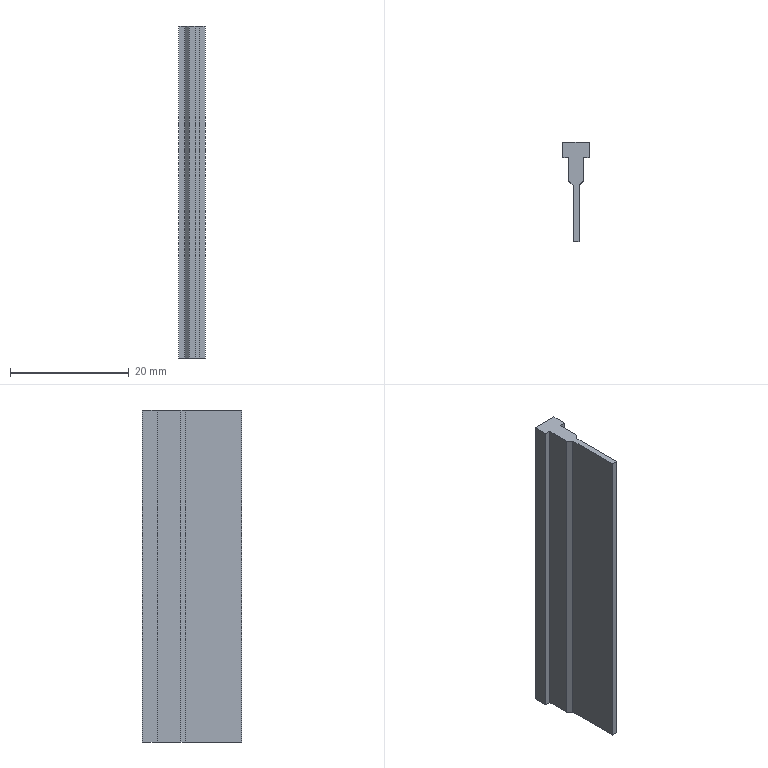Part | NX | features BREP 2 | 2 solids | 28 faces | box 4.458 x 16.702 x 56 mm | volume 3550 mm3 | plane 28
STEP:
#1=CARTESIAN_POINT('',(1.229,1.86,-4.));
#2=VERTEX_POINT('',#1);
#3=CARTESIAN_POINT('',(1.229,1.86,52.));
#4=VERTEX_POINT('',#3);
#5=CARTESIAN_POINT('',(1.229,1.86,0.));
#6=DIRECTION('',(0.,0.,1.));
#7=VECTOR('',#6,1000.);
#8=LINE('',#5,#7);
#9=EDGE_CURVE('',#2,#4,#8,.T.);
#10=ORIENTED_EDGE('',*,*,#9,.T.);
#11=CARTESIAN_POINT('',(0.521,1.152,52.));
#12=VERTEX_POINT('',#11);
#13=CARTESIAN_POINT('',(1.229,1.86,52.));
#14=DIRECTION('',(0.7071,0.7071,0.));
#15=VECTOR('',#14,1000.);
#16=LINE('',#13,#15);
#17=EDGE_CURVE('',#12,#4,#16,.T.);
#18=ORIENTED_EDGE('',*,*,#17,.F.);
#19=CARTESIAN_POINT('',(0.521,1.152,-4.));
#20=VERTEX_POINT('',#19);
#21=CARTESIAN_POINT('',(0.521,1.152,0.));
#22=DIRECTION('',(0.,0.,1.));
#23=VECTOR('',#22,1000.);
#24=LINE('',#21,#23);
#25=EDGE_CURVE('',#20,#12,#24,.T.);
#26=ORIENTED_EDGE('',*,*,#25,.F.);
#27=CARTESIAN_POINT('',(1.229,1.86,-4.));
#28=DIRECTION('',(0.7071,0.7071,0.));
#29=VECTOR('',#28,1000.);
#30=LINE('',#27,#29);
#31=EDGE_CURVE('',#20,#2,#30,.T.);
#32=ORIENTED_EDGE('',*,*,#31,.T.);
#33=EDGE_LOOP('',(#10,#18,#26,#32));
#34=FACE_BOUND('',#33,.T.);
#35=CARTESIAN_POINT('',(1.229,1.86,0.));
#36=DIRECTION('',(-0.7071,0.7071,0.));
#37=DIRECTION('',(0.7071,0.7071,0.));
#38=AXIS2_PLACEMENT_3D('',#35,#36,#37);
#39=PLANE('',#38);
#40=ADVANCED_FACE('',(#34),#39,.F.);
#41=CARTESIAN_POINT('',(0.521,-8.351,-4.));
#42=VERTEX_POINT('',#41);
#43=CARTESIAN_POINT('',(0.521,-8.351,52.));
#44=VERTEX_POINT('',#43);
#45=CARTESIAN_POINT('',(0.521,-8.351,0.));
#46=DIRECTION('',(0.,0.,1.));
#47=VECTOR('',#46,1000.);
#48=LINE('',#45,#47);
#49=EDGE_CURVE('',#42,#44,#48,.T.);
#50=ORIENTED_EDGE('',*,*,#49,.F.);
#51=CARTESIAN_POINT('',(0.521,-22.649,-4.));
#52=DIRECTION('',(0.,1.,0.));
#53=VECTOR('',#52,1000.);
#54=LINE('',#51,#53);
#55=EDGE_CURVE('',#42,#20,#54,.T.);
#56=ORIENTED_EDGE('',*,*,#55,.T.);
#57=ORIENTED_EDGE('',*,*,#25,.T.);
#58=CARTESIAN_POINT('',(0.521,-22.649,52.));
#59=DIRECTION('',(0.,1.,0.));
#60=VECTOR('',#59,1000.);
#61=LINE('',#58,#60);
#62=EDGE_CURVE('',#44,#12,#61,.T.);
#63=ORIENTED_EDGE('',*,*,#62,.F.);
#64=EDGE_LOOP('',(#50,#56,#57,#63));
#65=FACE_BOUND('',#64,.T.);
#66=CARTESIAN_POINT('',(0.521,-5.351,0.));
#67=DIRECTION('',(-1.,0.,0.));
#68=DIRECTION('',(0.,1.,0.));
#69=AXIS2_PLACEMENT_3D('',#66,#67,#68);
#70=PLANE('',#69);
#71=ADVANCED_FACE('',(#65),#70,.F.);
#72=ORIENTED_EDGE('',*,*,#49,.T.);
#73=CARTESIAN_POINT('',(-0.479,-8.351,52.));
#74=VERTEX_POINT('',#73);
#75=CARTESIAN_POINT('',(-3.521,-8.351,52.));
#76=DIRECTION('',(1.,0.,0.));
#77=VECTOR('',#76,1000.);
#78=LINE('',#75,#77);
#79=EDGE_CURVE('',#74,#44,#78,.T.);
#80=ORIENTED_EDGE('',*,*,#79,.F.);
#81=CARTESIAN_POINT('',(-0.479,-8.351,-4.));
#82=VERTEX_POINT('',#81);
#83=CARTESIAN_POINT('',(-0.479,-8.351,0.));
#84=DIRECTION('',(0.,0.,1.));
#85=VECTOR('',#84,1000.);
#86=LINE('',#83,#85);
#87=EDGE_CURVE('',#82,#74,#86,.T.);
#88=ORIENTED_EDGE('',*,*,#87,.F.);
#89=CARTESIAN_POINT('',(-3.521,-8.351,-4.));
#90=DIRECTION('',(1.,0.,0.));
#91=VECTOR('',#90,1000.);
#92=LINE('',#89,#91);
#93=EDGE_CURVE('',#82,#42,#92,.T.);
#94=ORIENTED_EDGE('',*,*,#93,.T.);
#95=EDGE_LOOP('',(#72,#80,#88,#94));
#96=FACE_BOUND('',#95,.T.);
#97=CARTESIAN_POINT('',(-3.521,-8.351,0.));
#98=DIRECTION('',(0.,-1.,0.));
#99=DIRECTION('',(-1.,0.,0.));
#100=AXIS2_PLACEMENT_3D('',#97,#98,#99);
#101=PLANE('',#100);
#102=ADVANCED_FACE('',(#96),#101,.T.);
#103=CARTESIAN_POINT('',(-0.479,1.107,-4.));
#104=VERTEX_POINT('',#103);
#105=CARTESIAN_POINT('',(-0.479,1.107,52.));
#106=VERTEX_POINT('',#105);
#107=CARTESIAN_POINT('',(-0.479,1.107,0.));
#108=DIRECTION('',(0.,0.,1.));
#109=VECTOR('',#108,1000.);
#110=LINE('',#107,#109);
#111=EDGE_CURVE('',#104,#106,#110,.T.);
#112=ORIENTED_EDGE('',*,*,#111,.F.);
#113=CARTESIAN_POINT('',(-0.479,-22.649,-4.));
#114=DIRECTION('',(0.,-1.,0.));
#115=VECTOR('',#114,1000.);
#116=LINE('',#113,#115);
#117=EDGE_CURVE('',#104,#82,#116,.T.);
#118=ORIENTED_EDGE('',*,*,#117,.T.);
#119=ORIENTED_EDGE('',*,*,#87,.T.);
#120=CARTESIAN_POINT('',(-0.479,-22.649,52.));
#121=DIRECTION('',(0.,-1.,0.));
#122=VECTOR('',#121,1000.);
#123=LINE('',#120,#122);
#124=EDGE_CURVE('',#106,#74,#123,.T.);
#125=ORIENTED_EDGE('',*,*,#124,.F.);
#126=EDGE_LOOP('',(#112,#118,#119,#125));
#127=FACE_BOUND('',#126,.T.);
#128=CARTESIAN_POINT('',(-0.479,-4.148,0.));
#129=DIRECTION('',(1.,0.,0.));
#130=DIRECTION('',(0.,-1.,0.));
#131=AXIS2_PLACEMENT_3D('',#128,#129,#130);
#132=PLANE('',#131);
#133=ADVANCED_FACE('',(#127),#132,.F.);
#134=ORIENTED_EDGE('',*,*,#111,.T.);
#135=CARTESIAN_POINT('',(-1.229,1.857,52.));
#136=VERTEX_POINT('',#135);
#137=CARTESIAN_POINT('',(-0.479,1.107,52.));
#138=DIRECTION('',(0.7071,-0.7071,0.));
#139=VECTOR('',#138,1000.);
#140=LINE('',#137,#139);
#141=EDGE_CURVE('',#136,#106,#140,.T.);
#142=ORIENTED_EDGE('',*,*,#141,.F.);
#143=CARTESIAN_POINT('',(-1.229,1.857,-4.));
#144=VERTEX_POINT('',#143);
#145=CARTESIAN_POINT('',(-1.229,1.857,0.));
#146=DIRECTION('',(0.,0.,1.));
#147=VECTOR('',#146,1000.);
#148=LINE('',#145,#147);
#149=EDGE_CURVE('',#144,#136,#148,.T.);
#150=ORIENTED_EDGE('',*,*,#149,.F.);
#151=CARTESIAN_POINT('',(-0.479,1.107,-4.));
#152=DIRECTION('',(0.7071,-0.7071,0.));
#153=VECTOR('',#152,1000.);
#154=LINE('',#151,#153);
#155=EDGE_CURVE('',#144,#104,#154,.T.);
#156=ORIENTED_EDGE('',*,*,#155,.T.);
#157=EDGE_LOOP('',(#134,#142,#150,#156));
#158=FACE_BOUND('',#157,.T.);
#159=CARTESIAN_POINT('',(-0.479,1.107,0.));
#160=DIRECTION('',(0.7071,0.7071,0.));
#161=DIRECTION('',(0.7071,-0.7071,0.));
#162=AXIS2_PLACEMENT_3D('',#159,#160,#161);
#163=PLANE('',#162);
#164=ADVANCED_FACE('',(#158),#163,.F.);
#165=ORIENTED_EDGE('',*,*,#149,.T.);
#166=CARTESIAN_POINT('',(-1.229,5.852,52.));
#167=VERTEX_POINT('',#166);
#168=CARTESIAN_POINT('',(-1.229,-22.649,52.));
#169=DIRECTION('',(0.,-1.,0.));
#170=VECTOR('',#169,1000.);
#171=LINE('',#168,#170);
#172=EDGE_CURVE('',#167,#136,#171,.T.);
#173=ORIENTED_EDGE('',*,*,#172,.F.);
#174=CARTESIAN_POINT('',(-1.229,5.852,-4.));
#175=VERTEX_POINT('',#174);
#176=CARTESIAN_POINT('',(-1.229,5.852,0.));
#177=DIRECTION('',(0.,0.,1.));
#178=VECTOR('',#177,1000.);
#179=LINE('',#176,#178);
#180=EDGE_CURVE('',#175,#167,#179,.T.);
#181=ORIENTED_EDGE('',*,*,#180,.F.);
#182=CARTESIAN_POINT('',(-1.229,-22.649,-4.));
#183=DIRECTION('',(0.,-1.,0.));
#184=VECTOR('',#183,1000.);
#185=LINE('',#182,#184);
#186=EDGE_CURVE('',#175,#144,#185,.T.);
#187=ORIENTED_EDGE('',*,*,#186,.T.);
#188=EDGE_LOOP('',(#165,#173,#181,#187));
#189=FACE_BOUND('',#188,.T.);
#190=CARTESIAN_POINT('',(-1.229,1.857,0.));
#191=DIRECTION('',(1.,0.,0.));
#192=DIRECTION('',(0.,-1.,0.));
#193=AXIS2_PLACEMENT_3D('',#190,#191,#192);
#194=PLANE('',#193);
#195=ADVANCED_FACE('',(#189),#194,.F.);
#196=ORIENTED_EDGE('',*,*,#180,.T.);
#197=CARTESIAN_POINT('',(-2.229,5.852,52.));
#198=VERTEX_POINT('',#197);
#199=CARTESIAN_POINT('',(-3.521,5.852,52.));
#200=DIRECTION('',(1.,0.,0.));
#201=VECTOR('',#200,1000.);
#202=LINE('',#199,#201);
#203=EDGE_CURVE('',#198,#167,#202,.T.);
#204=ORIENTED_EDGE('',*,*,#203,.F.);
#205=CARTESIAN_POINT('',(-2.229,5.852,-4.));
#206=VERTEX_POINT('',#205);
#207=CARTESIAN_POINT('',(-2.229,5.852,0.));
#208=DIRECTION('',(0.,0.,1.));
#209=VECTOR('',#208,1000.);
#210=LINE('',#207,#209);
#211=EDGE_CURVE('',#206,#198,#210,.T.);
#212=ORIENTED_EDGE('',*,*,#211,.F.);
#213=CARTESIAN_POINT('',(-3.521,5.852,-4.));
#214=DIRECTION('',(1.,0.,0.));
#215=VECTOR('',#214,1000.);
#216=LINE('',#213,#215);
#217=EDGE_CURVE('',#206,#175,#216,.T.);
#218=ORIENTED_EDGE('',*,*,#217,.T.);
#219=EDGE_LOOP('',(#196,#204,#212,#218));
#220=FACE_BOUND('',#219,.T.);
#221=CARTESIAN_POINT('',(-1.229,5.852,0.));
#222=DIRECTION('',(0.,1.,0.));
#223=DIRECTION('',(1.,0.,0.));
#224=AXIS2_PLACEMENT_3D('',#221,#222,#223);
#225=PLANE('',#224);
#226=ADVANCED_FACE('',(#220),#225,.F.);
#227=ORIENTED_EDGE('',*,*,#211,.T.);
#228=CARTESIAN_POINT('',(-2.229,8.351,52.));
#229=VERTEX_POINT('',#228);
#230=CARTESIAN_POINT('',(-2.229,-22.649,52.));
#231=DIRECTION('',(0.,-1.,0.));
#232=VECTOR('',#231,1000.);
#233=LINE('',#230,#232);
#234=EDGE_CURVE('',#229,#198,#233,.T.);
#235=ORIENTED_EDGE('',*,*,#234,.F.);
#236=CARTESIAN_POINT('',(-2.229,8.351,-4.));
#237=VERTEX_POINT('',#236);
#238=CARTESIAN_POINT('',(-2.229,8.351,0.));
#239=DIRECTION('',(0.,0.,1.));
#240=VECTOR('',#239,1000.);
#241=LINE('',#238,#240);
#242=EDGE_CURVE('',#237,#229,#241,.T.);
#243=ORIENTED_EDGE('',*,*,#242,.F.);
#244=CARTESIAN_POINT('',(-2.229,-22.649,-4.));
#245=DIRECTION('',(0.,-1.,0.));
#246=VECTOR('',#245,1000.);
#247=LINE('',#244,#246);
#248=EDGE_CURVE('',#237,#206,#247,.T.);
#249=ORIENTED_EDGE('',*,*,#248,.T.);
#250=EDGE_LOOP('',(#227,#235,#243,#249));
#251=FACE_BOUND('',#250,.T.);
#252=CARTESIAN_POINT('',(-2.229,-22.649,0.));
#253=DIRECTION('',(1.,0.,0.));
#254=DIRECTION('',(0.,-1.,0.));
#255=AXIS2_PLACEMENT_3D('',#252,#253,#254);
#256=PLANE('',#255);
#257=ADVANCED_FACE('',(#251),#256,.F.);
#258=ORIENTED_EDGE('',*,*,#242,.T.);
#259=CARTESIAN_POINT('',(2.229,8.351,52.));
#260=VERTEX_POINT('',#259);
#261=CARTESIAN_POINT('',(-3.521,8.351,52.));
#262=DIRECTION('',(-1.,0.,0.));
#263=VECTOR('',#262,1000.);
#264=LINE('',#261,#263);
#265=EDGE_CURVE('',#260,#229,#264,.T.);
#266=ORIENTED_EDGE('',*,*,#265,.F.);
#267=CARTESIAN_POINT('',(2.229,8.351,-4.));
#268=VERTEX_POINT('',#267);
#269=CARTESIAN_POINT('',(2.229,8.351,0.));
#270=DIRECTION('',(0.,0.,1.));
#271=VECTOR('',#270,1000.);
#272=LINE('',#269,#271);
#273=EDGE_CURVE('',#268,#260,#272,.T.);
#274=ORIENTED_EDGE('',*,*,#273,.F.);
#275=CARTESIAN_POINT('',(-3.521,8.351,-4.));
#276=DIRECTION('',(-1.,0.,0.));
#277=VECTOR('',#276,1000.);
#278=LINE('',#275,#277);
#279=EDGE_CURVE('',#268,#237,#278,.T.);
#280=ORIENTED_EDGE('',*,*,#279,.T.);
#281=EDGE_LOOP('',(#258,#266,#274,#280));
#282=FACE_BOUND('',#281,.T.);
#283=CARTESIAN_POINT('',(-25.771,8.351,0.));
#284=DIRECTION('',(0.,-1.,0.));
#285=DIRECTION('',(-1.,0.,0.));
#286=AXIS2_PLACEMENT_3D('',#283,#284,#285);
#287=PLANE('',#286);
#288=ADVANCED_FACE('',(#282),#287,.F.);
#289=ORIENTED_EDGE('',*,*,#273,.T.);
#290=CARTESIAN_POINT('',(2.229,5.852,52.));
#291=VERTEX_POINT('',#290);
#292=CARTESIAN_POINT('',(2.229,-22.649,52.));
#293=DIRECTION('',(0.,1.,0.));
#294=VECTOR('',#293,1000.);
#295=LINE('',#292,#294);
#296=EDGE_CURVE('',#291,#260,#295,.T.);
#297=ORIENTED_EDGE('',*,*,#296,.F.);
#298=CARTESIAN_POINT('',(2.229,5.852,-4.));
#299=VERTEX_POINT('',#298);
#300=CARTESIAN_POINT('',(2.229,5.852,0.));
#301=DIRECTION('',(0.,0.,1.));
#302=VECTOR('',#301,1000.);
#303=LINE('',#300,#302);
#304=EDGE_CURVE('',#299,#291,#303,.T.);
#305=ORIENTED_EDGE('',*,*,#304,.F.);
#306=CARTESIAN_POINT('',(2.229,-22.649,-4.));
#307=DIRECTION('',(0.,1.,0.));
#308=VECTOR('',#307,1000.);
#309=LINE('',#306,#308);
#310=EDGE_CURVE('',#299,#268,#309,.T.);
#311=ORIENTED_EDGE('',*,*,#310,.T.);
#312=EDGE_LOOP('',(#289,#297,#305,#311));
#313=FACE_BOUND('',#312,.T.);
#314=CARTESIAN_POINT('',(2.229,-22.649,0.));
#315=DIRECTION('',(1.,0.,0.));
#316=DIRECTION('',(0.,-1.,0.));
#317=AXIS2_PLACEMENT_3D('',#314,#315,#316);
#318=PLANE('',#317);
#319=ADVANCED_FACE('',(#313),#318,.T.);
#320=ORIENTED_EDGE('',*,*,#304,.T.);
#321=CARTESIAN_POINT('',(1.229,5.852,52.));
#322=VERTEX_POINT('',#321);
#323=CARTESIAN_POINT('',(-3.521,5.852,52.));
#324=DIRECTION('',(1.,0.,0.));
#325=VECTOR('',#324,1000.);
#326=LINE('',#323,#325);
#327=EDGE_CURVE('',#322,#291,#326,.T.);
#328=ORIENTED_EDGE('',*,*,#327,.F.);
#329=CARTESIAN_POINT('',(1.229,5.852,-4.));
#330=VERTEX_POINT('',#329);
#331=CARTESIAN_POINT('',(1.229,5.852,0.));
#332=DIRECTION('',(0.,0.,1.));
#333=VECTOR('',#332,1000.);
#334=LINE('',#331,#333);
#335=EDGE_CURVE('',#330,#322,#334,.T.);
#336=ORIENTED_EDGE('',*,*,#335,.F.);
#337=CARTESIAN_POINT('',(-3.521,5.852,-4.));
#338=DIRECTION('',(1.,0.,0.));
#339=VECTOR('',#338,1000.);
#340=LINE('',#337,#339);
#341=EDGE_CURVE('',#330,#299,#340,.T.);
#342=ORIENTED_EDGE('',*,*,#341,.T.);
#343=EDGE_LOOP('',(#320,#328,#336,#342));
#344=FACE_BOUND('',#343,.T.);
#345=CARTESIAN_POINT('',(2.229,5.852,0.));
#346=DIRECTION('',(0.,1.,0.));
#347=DIRECTION('',(1.,0.,0.));
#348=AXIS2_PLACEMENT_3D('',#345,#346,#347);
#349=PLANE('',#348);
#350=ADVANCED_FACE('',(#344),#349,.F.);
#351=CARTESIAN_POINT('',(1.229,-22.649,-4.));
#352=DIRECTION('',(0.,1.,0.));
#353=VECTOR('',#352,1000.);
#354=LINE('',#351,#353);
#355=EDGE_CURVE('',#2,#330,#354,.T.);
#356=ORIENTED_EDGE('',*,*,#355,.T.);
#357=ORIENTED_EDGE('',*,*,#335,.T.);
#358=CARTESIAN_POINT('',(1.229,-22.649,52.));
#359=DIRECTION('',(0.,1.,0.));
#360=VECTOR('',#359,1000.);
#361=LINE('',#358,#360);
#362=EDGE_CURVE('',#4,#322,#361,.T.);
#363=ORIENTED_EDGE('',*,*,#362,.F.);
#364=ORIENTED_EDGE('',*,*,#9,.F.);
#365=EDGE_LOOP('',(#356,#357,#363,#364));
#366=FACE_BOUND('',#365,.T.);
#367=CARTESIAN_POINT('',(1.229,5.852,0.));
#368=DIRECTION('',(-1.,0.,0.));
#369=DIRECTION('',(0.,1.,0.));
#370=AXIS2_PLACEMENT_3D('',#367,#368,#369);
#371=PLANE('',#370);
#372=ADVANCED_FACE('',(#366),#371,.F.);
#373=ORIENTED_EDGE('',*,*,#327,.T.);
#374=ORIENTED_EDGE('',*,*,#296,.T.);
#375=ORIENTED_EDGE('',*,*,#265,.T.);
#376=ORIENTED_EDGE('',*,*,#234,.T.);
#377=ORIENTED_EDGE('',*,*,#203,.T.);
#378=ORIENTED_EDGE('',*,*,#172,.T.);
#379=ORIENTED_EDGE('',*,*,#141,.T.);
#380=ORIENTED_EDGE('',*,*,#124,.T.);
#381=ORIENTED_EDGE('',*,*,#79,.T.);
#382=ORIENTED_EDGE('',*,*,#62,.T.);
#383=ORIENTED_EDGE('',*,*,#17,.T.);
#384=ORIENTED_EDGE('',*,*,#362,.T.);
#385=EDGE_LOOP('',(#373,#374,#375,#376,#377,#378,#379,#380,#381,#382,#383,#384));
#386=FACE_BOUND('',#385,.T.);
#387=CARTESIAN_POINT('',(-3.521,-22.649,52.));
#388=DIRECTION('',(0.,0.,1.));
#389=DIRECTION('',(-1.,0.,0.));
#390=AXIS2_PLACEMENT_3D('',#387,#388,#389);
#391=PLANE('',#390);
#392=ADVANCED_FACE('',(#386),#391,.T.);
#393=ORIENTED_EDGE('',*,*,#341,.F.);
#394=ORIENTED_EDGE('',*,*,#355,.F.);
#395=ORIENTED_EDGE('',*,*,#31,.F.);
#396=ORIENTED_EDGE('',*,*,#55,.F.);
#397=ORIENTED_EDGE('',*,*,#93,.F.);
#398=ORIENTED_EDGE('',*,*,#117,.F.);
#399=ORIENTED_EDGE('',*,*,#155,.F.);
#400=ORIENTED_EDGE('',*,*,#186,.F.);
#401=ORIENTED_EDGE('',*,*,#217,.F.);
#402=ORIENTED_EDGE('',*,*,#248,.F.);
#403=ORIENTED_EDGE('',*,*,#279,.F.);
#404=ORIENTED_EDGE('',*,*,#310,.F.);
#405=EDGE_LOOP('',(#393,#394,#395,#396,#397,#398,#399,#400,#401,#402,#403,#404));
#406=FACE_BOUND('',#405,.T.);
#407=CARTESIAN_POINT('',(-3.521,-22.649,-4.));
#408=DIRECTION('',(0.,0.,1.));
#409=DIRECTION('',(-1.,0.,0.));
#410=AXIS2_PLACEMENT_3D('',#407,#408,#409);
#411=PLANE('',#410);
#412=ADVANCED_FACE('',(#406),#411,.F.);
#413=CLOSED_SHELL('',(#40,#71,#102,#133,#164,#195,#226,#257,#288,#319,#350,#372,#392,#412));
#414=MANIFOLD_SOLID_BREP('',#413);
#415=CARTESIAN_POINT('',(1.229,1.86,-4.));
#416=VERTEX_POINT('',#415);
#417=CARTESIAN_POINT('',(1.229,1.86,52.));
#418=VERTEX_POINT('',#417);
#419=CARTESIAN_POINT('',(1.229,1.86,0.));
#420=DIRECTION('',(0.,0.,1.));
#421=VECTOR('',#420,1000.);
#422=LINE('',#419,#421);
#423=EDGE_CURVE('',#416,#418,#422,.T.);
#424=ORIENTED_EDGE('',*,*,#423,.T.);
#425=CARTESIAN_POINT('',(0.521,1.152,52.));
#426=VERTEX_POINT('',#425);
#427=CARTESIAN_POINT('',(1.229,1.86,52.));
#428=DIRECTION('',(0.7071,0.7071,0.));
#429=VECTOR('',#428,1000.);
#430=LINE('',#427,#429);
#431=EDGE_CURVE('',#426,#418,#430,.T.);
#432=ORIENTED_EDGE('',*,*,#431,.F.);
#433=CARTESIAN_POINT('',(0.521,1.152,-4.));
#434=VERTEX_POINT('',#433);
#435=CARTESIAN_POINT('',(0.521,1.152,0.));
#436=DIRECTION('',(0.,0.,1.));
#437=VECTOR('',#436,1000.);
#438=LINE('',#435,#437);
#439=EDGE_CURVE('',#434,#426,#438,.T.);
#440=ORIENTED_EDGE('',*,*,#439,.F.);
#441=CARTESIAN_POINT('',(1.229,1.86,-4.));
#442=DIRECTION('',(0.7071,0.7071,0.));
#443=VECTOR('',#442,1000.);
#444=LINE('',#441,#443);
#445=EDGE_CURVE('',#434,#416,#444,.T.);
#446=ORIENTED_EDGE('',*,*,#445,.T.);
#447=EDGE_LOOP('',(#424,#432,#440,#446));
#448=FACE_BOUND('',#447,.T.);
#449=CARTESIAN_POINT('',(1.229,1.86,0.));
#450=DIRECTION('',(-0.7071,0.7071,0.));
#451=DIRECTION('',(0.7071,0.7071,0.));
#452=AXIS2_PLACEMENT_3D('',#449,#450,#451);
#453=PLANE('',#452);
#454=ADVANCED_FACE('',(#448),#453,.F.);
#455=CARTESIAN_POINT('',(0.521,-8.351,-4.));
#456=VERTEX_POINT('',#455);
#457=CARTESIAN_POINT('',(0.521,-8.351,52.));
#458=VERTEX_POINT('',#457);
#459=CARTESIAN_POINT('',(0.521,-8.351,0.));
#460=DIRECTION('',(0.,0.,1.));
#461=VECTOR('',#460,1000.);
#462=LINE('',#459,#461);
#463=EDGE_CURVE('',#456,#458,#462,.T.);
#464=ORIENTED_EDGE('',*,*,#463,.F.);
#465=CARTESIAN_POINT('',(0.521,-22.649,-4.));
#466=DIRECTION('',(0.,1.,0.));
#467=VECTOR('',#466,1000.);
#468=LINE('',#465,#467);
#469=EDGE_CURVE('',#456,#434,#468,.T.);
#470=ORIENTED_EDGE('',*,*,#469,.T.);
#471=ORIENTED_EDGE('',*,*,#439,.T.);
#472=CARTESIAN_POINT('',(0.521,-22.649,52.));
#473=DIRECTION('',(0.,1.,0.));
#474=VECTOR('',#473,1000.);
#475=LINE('',#472,#474);
#476=EDGE_CURVE('',#458,#426,#475,.T.);
#477=ORIENTED_EDGE('',*,*,#476,.F.);
#478=EDGE_LOOP('',(#464,#470,#471,#477));
#479=FACE_BOUND('',#478,.T.);
#480=CARTESIAN_POINT('',(0.521,-5.351,0.));
#481=DIRECTION('',(-1.,0.,0.));
#482=DIRECTION('',(0.,1.,0.));
#483=AXIS2_PLACEMENT_3D('',#480,#481,#482);
#484=PLANE('',#483);
#485=ADVANCED_FACE('',(#479),#484,.F.);
#486=ORIENTED_EDGE('',*,*,#463,.T.);
#487=CARTESIAN_POINT('',(-0.479,-8.351,52.));
#488=VERTEX_POINT('',#487);
#489=CARTESIAN_POINT('',(-3.521,-8.351,52.));
#490=DIRECTION('',(1.,0.,0.));
#491=VECTOR('',#490,1000.);
#492=LINE('',#489,#491);
#493=EDGE_CURVE('',#488,#458,#492,.T.);
#494=ORIENTED_EDGE('',*,*,#493,.F.);
#495=CARTESIAN_POINT('',(-0.479,-8.351,-4.));
#496=VERTEX_POINT('',#495);
#497=CARTESIAN_POINT('',(-0.479,-8.351,0.));
#498=DIRECTION('',(0.,0.,1.));
#499=VECTOR('',#498,1000.);
#500=LINE('',#497,#499);
#501=EDGE_CURVE('',#496,#488,#500,.T.);
#502=ORIENTED_EDGE('',*,*,#501,.F.);
#503=CARTESIAN_POINT('',(-3.521,-8.351,-4.));
#504=DIRECTION('',(1.,0.,0.));
#505=VECTOR('',#504,1000.);
#506=LINE('',#503,#505);
#507=EDGE_CURVE('',#496,#456,#506,.T.);
#508=ORIENTED_EDGE('',*,*,#507,.T.);
#509=EDGE_LOOP('',(#486,#494,#502,#508));
#510=FACE_BOUND('',#509,.T.);
#511=CARTESIAN_POINT('',(-3.521,-8.351,0.));
#512=DIRECTION('',(0.,-1.,0.));
#513=DIRECTION('',(-1.,0.,0.));
#514=AXIS2_PLACEMENT_3D('',#511,#512,#513);
#515=PLANE('',#514);
#516=ADVANCED_FACE('',(#510),#515,.T.);
#517=CARTESIAN_POINT('',(-0.479,1.107,-4.));
#518=VERTEX_POINT('',#517);
#519=CARTESIAN_POINT('',(-0.479,1.107,52.));
#520=VERTEX_POINT('',#519);
#521=CARTESIAN_POINT('',(-0.479,1.107,0.));
#522=DIRECTION('',(0.,0.,1.));
#523=VECTOR('',#522,1000.);
#524=LINE('',#521,#523);
#525=EDGE_CURVE('',#518,#520,#524,.T.);
#526=ORIENTED_EDGE('',*,*,#525,.F.);
#527=CARTESIAN_POINT('',(-0.479,-22.649,-4.));
#528=DIRECTION('',(0.,-1.,0.));
#529=VECTOR('',#528,1000.);
#530=LINE('',#527,#529);
#531=EDGE_CURVE('',#518,#496,#530,.T.);
#532=ORIENTED_EDGE('',*,*,#531,.T.);
#533=ORIENTED_EDGE('',*,*,#501,.T.);
#534=CARTESIAN_POINT('',(-0.479,-22.649,52.));
#535=DIRECTION('',(0.,-1.,0.));
#536=VECTOR('',#535,1000.);
#537=LINE('',#534,#536);
#538=EDGE_CURVE('',#520,#488,#537,.T.);
#539=ORIENTED_EDGE('',*,*,#538,.F.);
#540=EDGE_LOOP('',(#526,#532,#533,#539));
#541=FACE_BOUND('',#540,.T.);
#542=CARTESIAN_POINT('',(-0.479,-4.148,0.));
#543=DIRECTION('',(1.,0.,0.));
#544=DIRECTION('',(0.,-1.,0.));
#545=AXIS2_PLACEMENT_3D('',#542,#543,#544);
#546=PLANE('',#545);
#547=ADVANCED_FACE('',(#541),#546,.F.);
#548=ORIENTED_EDGE('',*,*,#525,.T.);
#549=CARTESIAN_POINT('',(-1.229,1.857,52.));
#550=VERTEX_POINT('',#549);
#551=CARTESIAN_POINT('',(-0.479,1.107,52.));
#552=DIRECTION('',(0.7071,-0.7071,0.));
#553=VECTOR('',#552,1000.);
#554=LINE('',#551,#553);
#555=EDGE_CURVE('',#550,#520,#554,.T.);
#556=ORIENTED_EDGE('',*,*,#555,.F.);
#557=CARTESIAN_POINT('',(-1.229,1.857,-4.));
#558=VERTEX_POINT('',#557);
#559=CARTESIAN_POINT('',(-1.229,1.857,0.));
#560=DIRECTION('',(0.,0.,1.));
#561=VECTOR('',#560,1000.);
#562=LINE('',#559,#561);
#563=EDGE_CURVE('',#558,#550,#562,.T.);
#564=ORIENTED_EDGE('',*,*,#563,.F.);
#565=CARTESIAN_POINT('',(-0.479,1.107,-4.));
#566=DIRECTION('',(0.7071,-0.7071,0.));
#567=VECTOR('',#566,1000.);
#568=LINE('',#565,#567);
#569=EDGE_CURVE('',#558,#518,#568,.T.);
#570=ORIENTED_EDGE('',*,*,#569,.T.);
#571=EDGE_LOOP('',(#548,#556,#564,#570));
#572=FACE_BOUND('',#571,.T.);
#573=CARTESIAN_POINT('',(-0.479,1.107,0.));
#574=DIRECTION('',(0.7071,0.7071,0.));
#575=DIRECTION('',(0.7071,-0.7071,0.));
#576=AXIS2_PLACEMENT_3D('',#573,#574,#575);
#577=PLANE('',#576);
#578=ADVANCED_FACE('',(#572),#577,.F.);
#579=ORIENTED_EDGE('',*,*,#563,.T.);
#580=CARTESIAN_POINT('',(-1.229,5.852,52.));
#581=VERTEX_POINT('',#580);
#582=CARTESIAN_POINT('',(-1.229,-22.649,52.));
#583=DIRECTION('',(0.,-1.,0.));
#584=VECTOR('',#583,1000.);
#585=LINE('',#582,#584);
#586=EDGE_CURVE('',#581,#550,#585,.T.);
#587=ORIENTED_EDGE('',*,*,#586,.F.);
#588=CARTESIAN_POINT('',(-1.229,5.852,-4.));
#589=VERTEX_POINT('',#588);
#590=CARTESIAN_POINT('',(-1.229,5.852,0.));
#591=DIRECTION('',(0.,0.,1.));
#592=VECTOR('',#591,1000.);
#593=LINE('',#590,#592);
#594=EDGE_CURVE('',#589,#581,#593,.T.);
#595=ORIENTED_EDGE('',*,*,#594,.F.);
#596=CARTESIAN_POINT('',(-1.229,-22.649,-4.));
#597=DIRECTION('',(0.,-1.,0.));
#598=VECTOR('',#597,1000.);
#599=LINE('',#596,#598);
#600=EDGE_CURVE('',#589,#558,#599,.T.);
#601=ORIENTED_EDGE('',*,*,#600,.T.);
#602=EDGE_LOOP('',(#579,#587,#595,#601));
#603=FACE_BOUND('',#602,.T.);
#604=CARTESIAN_POINT('',(-1.229,1.857,0.));
#605=DIRECTION('',(1.,0.,0.));
#606=DIRECTION('',(0.,-1.,0.));
#607=AXIS2_PLACEMENT_3D('',#604,#605,#606);
#608=PLANE('',#607);
#609=ADVANCED_FACE('',(#603),#608,.F.);
#610=ORIENTED_EDGE('',*,*,#594,.T.);
#611=CARTESIAN_POINT('',(-2.229,5.852,52.));
#612=VERTEX_POINT('',#611);
#613=CARTESIAN_POINT('',(-3.521,5.852,52.));
#614=DIRECTION('',(1.,0.,0.));
#615=VECTOR('',#614,1000.);
#616=LINE('',#613,#615);
#617=EDGE_CURVE('',#612,#581,#616,.T.);
#618=ORIENTED_EDGE('',*,*,#617,.F.);
#619=CARTESIAN_POINT('',(-2.229,5.852,-4.));
#620=VERTEX_POINT('',#619);
#621=CARTESIAN_POINT('',(-2.229,5.852,0.));
#622=DIRECTION('',(0.,0.,1.));
#623=VECTOR('',#622,1000.);
#624=LINE('',#621,#623);
#625=EDGE_CURVE('',#620,#612,#624,.T.);
#626=ORIENTED_EDGE('',*,*,#625,.F.);
#627=CARTESIAN_POINT('',(-3.521,5.852,-4.));
#628=DIRECTION('',(1.,0.,0.));
#629=VECTOR('',#628,1000.);
#630=LINE('',#627,#629);
#631=EDGE_CURVE('',#620,#589,#630,.T.);
#632=ORIENTED_EDGE('',*,*,#631,.T.);
#633=EDGE_LOOP('',(#610,#618,#626,#632));
#634=FACE_BOUND('',#633,.T.);
#635=CARTESIAN_POINT('',(-1.229,5.852,0.));
#636=DIRECTION('',(0.,1.,0.));
#637=DIRECTION('',(1.,0.,0.));
#638=AXIS2_PLACEMENT_3D('',#635,#636,#637);
#639=PLANE('',#638);
#640=ADVANCED_FACE('',(#634),#639,.F.);
#641=ORIENTED_EDGE('',*,*,#625,.T.);
#642=CARTESIAN_POINT('',(-2.229,8.351,52.));
#643=VERTEX_POINT('',#642);
#644=CARTESIAN_POINT('',(-2.229,-22.649,52.));
#645=DIRECTION('',(0.,-1.,0.));
#646=VECTOR('',#645,1000.);
#647=LINE('',#644,#646);
#648=EDGE_CURVE('',#643,#612,#647,.T.);
#649=ORIENTED_EDGE('',*,*,#648,.F.);
#650=CARTESIAN_POINT('',(-2.229,8.351,-4.));
#651=VERTEX_POINT('',#650);
#652=CARTESIAN_POINT('',(-2.229,8.351,0.));
#653=DIRECTION('',(0.,0.,1.));
#654=VECTOR('',#653,1000.);
#655=LINE('',#652,#654);
#656=EDGE_CURVE('',#651,#643,#655,.T.);
#657=ORIENTED_EDGE('',*,*,#656,.F.);
#658=CARTESIAN_POINT('',(-2.229,-22.649,-4.));
#659=DIRECTION('',(0.,-1.,0.));
#660=VECTOR('',#659,1000.);
#661=LINE('',#658,#660);
#662=EDGE_CURVE('',#651,#620,#661,.T.);
#663=ORIENTED_EDGE('',*,*,#662,.T.);
#664=EDGE_LOOP('',(#641,#649,#657,#663));
#665=FACE_BOUND('',#664,.T.);
#666=CARTESIAN_POINT('',(-2.229,-22.649,0.));
#667=DIRECTION('',(1.,0.,0.));
#668=DIRECTION('',(0.,-1.,0.));
#669=AXIS2_PLACEMENT_3D('',#666,#667,#668);
#670=PLANE('',#669);
#671=ADVANCED_FACE('',(#665),#670,.F.);
#672=ORIENTED_EDGE('',*,*,#656,.T.);
#673=CARTESIAN_POINT('',(2.229,8.351,52.));
#674=VERTEX_POINT('',#673);
#675=CARTESIAN_POINT('',(-3.521,8.351,52.));
#676=DIRECTION('',(-1.,0.,0.));
#677=VECTOR('',#676,1000.);
#678=LINE('',#675,#677);
#679=EDGE_CURVE('',#674,#643,#678,.T.);
#680=ORIENTED_EDGE('',*,*,#679,.F.);
#681=CARTESIAN_POINT('',(2.229,8.351,-4.));
#682=VERTEX_POINT('',#681);
#683=CARTESIAN_POINT('',(2.229,8.351,0.));
#684=DIRECTION('',(0.,0.,1.));
#685=VECTOR('',#684,1000.);
#686=LINE('',#683,#685);
#687=EDGE_CURVE('',#682,#674,#686,.T.);
#688=ORIENTED_EDGE('',*,*,#687,.F.);
#689=CARTESIAN_POINT('',(-3.521,8.351,-4.));
#690=DIRECTION('',(-1.,0.,0.));
#691=VECTOR('',#690,1000.);
#692=LINE('',#689,#691);
#693=EDGE_CURVE('',#682,#651,#692,.T.);
#694=ORIENTED_EDGE('',*,*,#693,.T.);
#695=EDGE_LOOP('',(#672,#680,#688,#694));
#696=FACE_BOUND('',#695,.T.);
#697=CARTESIAN_POINT('',(-25.771,8.351,0.));
#698=DIRECTION('',(0.,-1.,0.));
#699=DIRECTION('',(-1.,0.,0.));
#700=AXIS2_PLACEMENT_3D('',#697,#698,#699);
#701=PLANE('',#700);
#702=ADVANCED_FACE('',(#696),#701,.F.);
#703=ORIENTED_EDGE('',*,*,#687,.T.);
#704=CARTESIAN_POINT('',(2.229,5.852,52.));
#705=VERTEX_POINT('',#704);
#706=CARTESIAN_POINT('',(2.229,-22.649,52.));
#707=DIRECTION('',(0.,1.,0.));
#708=VECTOR('',#707,1000.);
#709=LINE('',#706,#708);
#710=EDGE_CURVE('',#705,#674,#709,.T.);
#711=ORIENTED_EDGE('',*,*,#710,.F.);
#712=CARTESIAN_POINT('',(2.229,5.852,-4.));
#713=VERTEX_POINT('',#712);
#714=CARTESIAN_POINT('',(2.229,5.852,0.));
#715=DIRECTION('',(0.,0.,1.));
#716=VECTOR('',#715,1000.);
#717=LINE('',#714,#716);
#718=EDGE_CURVE('',#713,#705,#717,.T.);
#719=ORIENTED_EDGE('',*,*,#718,.F.);
#720=CARTESIAN_POINT('',(2.229,-22.649,-4.));
#721=DIRECTION('',(0.,1.,0.));
#722=VECTOR('',#721,1000.);
#723=LINE('',#720,#722);
#724=EDGE_CURVE('',#713,#682,#723,.T.);
#725=ORIENTED_EDGE('',*,*,#724,.T.);
#726=EDGE_LOOP('',(#703,#711,#719,#725));
#727=FACE_BOUND('',#726,.T.);
#728=CARTESIAN_POINT('',(2.229,-22.649,0.));
#729=DIRECTION('',(1.,0.,0.));
#730=DIRECTION('',(0.,-1.,0.));
#731=AXIS2_PLACEMENT_3D('',#728,#729,#730);
#732=PLANE('',#731);
#733=ADVANCED_FACE('',(#727),#732,.T.);
#734=ORIENTED_EDGE('',*,*,#718,.T.);
#735=CARTESIAN_POINT('',(1.229,5.852,52.));
#736=VERTEX_POINT('',#735);
#737=CARTESIAN_POINT('',(-3.521,5.852,52.));
#738=DIRECTION('',(1.,0.,0.));
#739=VECTOR('',#738,1000.);
#740=LINE('',#737,#739);
#741=EDGE_CURVE('',#736,#705,#740,.T.);
#742=ORIENTED_EDGE('',*,*,#741,.F.);
#743=CARTESIAN_POINT('',(1.229,5.852,-4.));
#744=VERTEX_POINT('',#743);
#745=CARTESIAN_POINT('',(1.229,5.852,0.));
#746=DIRECTION('',(0.,0.,1.));
#747=VECTOR('',#746,1000.);
#748=LINE('',#745,#747);
#749=EDGE_CURVE('',#744,#736,#748,.T.);
#750=ORIENTED_EDGE('',*,*,#749,.F.);
#751=CARTESIAN_POINT('',(-3.521,5.852,-4.));
#752=DIRECTION('',(1.,0.,0.));
#753=VECTOR('',#752,1000.);
#754=LINE('',#751,#753);
#755=EDGE_CURVE('',#744,#713,#754,.T.);
#756=ORIENTED_EDGE('',*,*,#755,.T.);
#757=EDGE_LOOP('',(#734,#742,#750,#756));
#758=FACE_BOUND('',#757,.T.);
#759=CARTESIAN_POINT('',(2.229,5.852,0.));
#760=DIRECTION('',(0.,1.,0.));
#761=DIRECTION('',(1.,0.,0.));
#762=AXIS2_PLACEMENT_3D('',#759,#760,#761);
#763=PLANE('',#762);
#764=ADVANCED_FACE('',(#758),#763,.F.);
#765=CARTESIAN_POINT('',(1.229,-22.649,-4.));
#766=DIRECTION('',(0.,1.,0.));
#767=VECTOR('',#766,1000.);
#768=LINE('',#765,#767);
#769=EDGE_CURVE('',#416,#744,#768,.T.);
#770=ORIENTED_EDGE('',*,*,#769,.T.);
#771=ORIENTED_EDGE('',*,*,#749,.T.);
#772=CARTESIAN_POINT('',(1.229,-22.649,52.));
#773=DIRECTION('',(0.,1.,0.));
#774=VECTOR('',#773,1000.);
#775=LINE('',#772,#774);
#776=EDGE_CURVE('',#418,#736,#775,.T.);
#777=ORIENTED_EDGE('',*,*,#776,.F.);
#778=ORIENTED_EDGE('',*,*,#423,.F.);
#779=EDGE_LOOP('',(#770,#771,#777,#778));
#780=FACE_BOUND('',#779,.T.);
#781=CARTESIAN_POINT('',(1.229,5.852,0.));
#782=DIRECTION('',(-1.,0.,0.));
#783=DIRECTION('',(0.,1.,0.));
#784=AXIS2_PLACEMENT_3D('',#781,#782,#783);
#785=PLANE('',#784);
#786=ADVANCED_FACE('',(#780),#785,.F.);
#787=ORIENTED_EDGE('',*,*,#741,.T.);
#788=ORIENTED_EDGE('',*,*,#710,.T.);
#789=ORIENTED_EDGE('',*,*,#679,.T.);
#790=ORIENTED_EDGE('',*,*,#648,.T.);
#791=ORIENTED_EDGE('',*,*,#617,.T.);
#792=ORIENTED_EDGE('',*,*,#586,.T.);
#793=ORIENTED_EDGE('',*,*,#555,.T.);
#794=ORIENTED_EDGE('',*,*,#538,.T.);
#795=ORIENTED_EDGE('',*,*,#493,.T.);
#796=ORIENTED_EDGE('',*,*,#476,.T.);
#797=ORIENTED_EDGE('',*,*,#431,.T.);
#798=ORIENTED_EDGE('',*,*,#776,.T.);
#799=EDGE_LOOP('',(#787,#788,#789,#790,#791,#792,#793,#794,#795,#796,#797,#798));
#800=FACE_BOUND('',#799,.T.);
#801=CARTESIAN_POINT('',(-3.521,-22.649,52.));
#802=DIRECTION('',(0.,0.,1.));
#803=DIRECTION('',(-1.,0.,0.));
#804=AXIS2_PLACEMENT_3D('',#801,#802,#803);
#805=PLANE('',#804);
#806=ADVANCED_FACE('',(#800),#805,.T.);
#807=ORIENTED_EDGE('',*,*,#755,.F.);
#808=ORIENTED_EDGE('',*,*,#769,.F.);
#809=ORIENTED_EDGE('',*,*,#445,.F.);
#810=ORIENTED_EDGE('',*,*,#469,.F.);
#811=ORIENTED_EDGE('',*,*,#507,.F.);
#812=ORIENTED_EDGE('',*,*,#531,.F.);
#813=ORIENTED_EDGE('',*,*,#569,.F.);
#814=ORIENTED_EDGE('',*,*,#600,.F.);
#815=ORIENTED_EDGE('',*,*,#631,.F.);
#816=ORIENTED_EDGE('',*,*,#662,.F.);
#817=ORIENTED_EDGE('',*,*,#693,.F.);
#818=ORIENTED_EDGE('',*,*,#724,.F.);
#819=EDGE_LOOP('',(#807,#808,#809,#810,#811,#812,#813,#814,#815,#816,#817,#818));
#820=FACE_BOUND('',#819,.T.);
#821=CARTESIAN_POINT('',(-3.521,-22.649,-4.));
#822=DIRECTION('',(0.,0.,1.));
#823=DIRECTION('',(-1.,0.,0.));
#824=AXIS2_PLACEMENT_3D('',#821,#822,#823);
#825=PLANE('',#824);
#826=ADVANCED_FACE('',(#820),#825,.F.);
#827=CLOSED_SHELL('',(#454,#485,#516,#547,#578,#609,#640,#671,#702,#733,#764,#786,#806,#826));
#828=MANIFOLD_SOLID_BREP('',#827);
#829=(LENGTH_UNIT()NAMED_UNIT(*)SI_UNIT(.MILLI.,.METRE.));
#830=UNCERTAINTY_MEASURE_WITH_UNIT(LENGTH_MEASURE(0.00001),#829,'','');
#831=(NAMED_UNIT(*)PLANE_ANGLE_UNIT()SI_UNIT($,.RADIAN.));
#832=(NAMED_UNIT(*)SI_UNIT($,.STERADIAN.)SOLID_ANGLE_UNIT());
#833=(GEOMETRIC_REPRESENTATION_CONTEXT(3)GLOBAL_UNCERTAINTY_ASSIGNED_CONTEXT((#830))GLOBAL_UNIT_ASSIGNED_CONTEXT((#829,#831,#832))REPRESENTATION_CONTEXT('',''));
#834=ADVANCED_BREP_SHAPE_REPRESENTATION('',(#414,#828),#833);